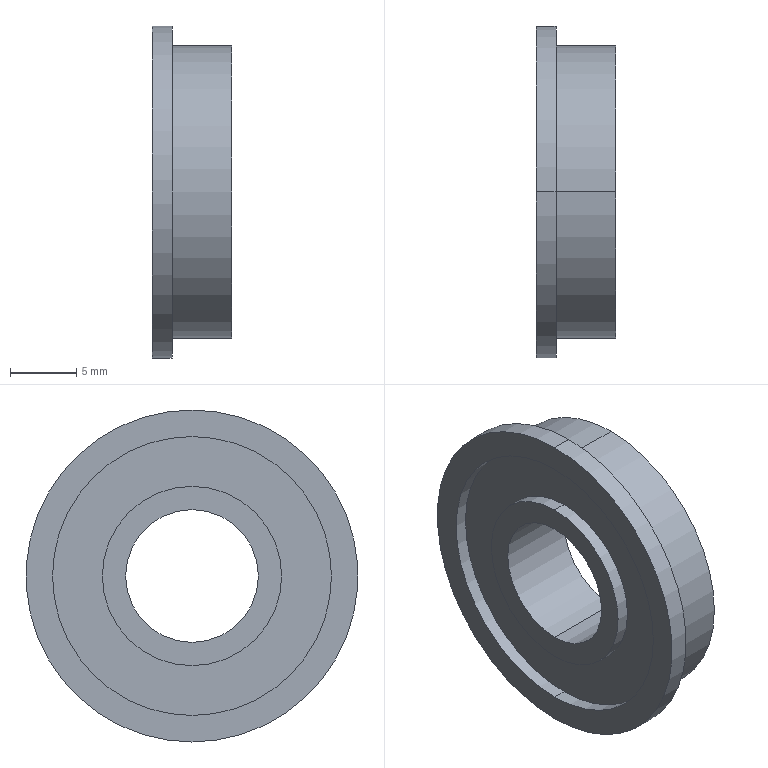Part | SolidWorks | features Stock 1 | 1 solid | 21 faces | box 6 x 25 x 25 mm | volume 1569 mm3 | cylinder 14 | plane 7 | commonest cylinder face diameters 13.5 x4 21 x4 10 x2 22 x2 25 x2
STEP:
#1=CARTESIAN_POINT('',(1.,0.,6.75));
#2=VERTEX_POINT('',#1);
#3=CARTESIAN_POINT('',(1.,0.,-6.75));
#4=VERTEX_POINT('',#3);
#5=CARTESIAN_POINT('',(1.,0.,0.));
#6=DIRECTION('',(-1.,0.,0.));
#7=DIRECTION('',(0.,0.,1.));
#8=AXIS2_PLACEMENT_3D('',#5,#6,#7);
#9=CIRCLE('',#8,6.75);
#10=EDGE_CURVE('',#2,#4,#9,.T.);
#11=ORIENTED_EDGE('',*,*,#10,.T.);
#12=CARTESIAN_POINT('',(0.,0.,-6.75));
#13=VERTEX_POINT('',#12);
#14=CARTESIAN_POINT('',(1.,0.,-6.75));
#15=DIRECTION('',(-1.,0.,0.));
#16=VECTOR('',#15,1000.);
#17=LINE('',#14,#16);
#18=EDGE_CURVE('',#4,#13,#17,.T.);
#19=ORIENTED_EDGE('',*,*,#18,.T.);
#20=CARTESIAN_POINT('',(0.,0.,6.75));
#21=VERTEX_POINT('',#20);
#22=CARTESIAN_POINT('',(0.,0.,0.));
#23=DIRECTION('',(-1.,0.,0.));
#24=DIRECTION('',(0.,0.,1.));
#25=AXIS2_PLACEMENT_3D('',#22,#23,#24);
#26=CIRCLE('',#25,6.75);
#27=EDGE_CURVE('',#21,#13,#26,.T.);
#28=ORIENTED_EDGE('',*,*,#27,.F.);
#29=CARTESIAN_POINT('',(1.,0.,6.75));
#30=DIRECTION('',(-1.,0.,0.));
#31=VECTOR('',#30,1000.);
#32=LINE('',#29,#31);
#33=EDGE_CURVE('',#2,#21,#32,.T.);
#34=ORIENTED_EDGE('',*,*,#33,.F.);
#35=EDGE_LOOP('',(#11,#19,#28,#34));
#36=FACE_OUTER_BOUND('',#35,.T.);
#37=CARTESIAN_POINT('',(1.,0.,0.));
#38=DIRECTION('',(-1.,0.,0.));
#39=DIRECTION('',(0.,0.,1.));
#40=AXIS2_PLACEMENT_3D('',#37,#38,#39);
#41=CYLINDRICAL_SURFACE('',#40,6.75);
#42=ADVANCED_FACE('',(#36),#41,.T.);
#43=CARTESIAN_POINT('',(1.,0.,-10.5));
#44=VERTEX_POINT('',#43);
#45=CARTESIAN_POINT('',(1.,0.,10.5));
#46=VERTEX_POINT('',#45);
#47=CARTESIAN_POINT('',(1.,0.,0.));
#48=DIRECTION('',(-1.,0.,0.));
#49=DIRECTION('',(0.,0.,1.));
#50=AXIS2_PLACEMENT_3D('',#47,#48,#49);
#51=CIRCLE('',#50,10.5);
#52=EDGE_CURVE('',#44,#46,#51,.T.);
#53=ORIENTED_EDGE('',*,*,#52,.F.);
#54=CARTESIAN_POINT('',(0.,0.,-10.5));
#55=VERTEX_POINT('',#54);
#56=CARTESIAN_POINT('',(1.,0.,-10.5));
#57=DIRECTION('',(-1.,0.,0.));
#58=VECTOR('',#57,1000.);
#59=LINE('',#56,#58);
#60=EDGE_CURVE('',#44,#55,#59,.T.);
#61=ORIENTED_EDGE('',*,*,#60,.T.);
#62=CARTESIAN_POINT('',(0.,0.,10.5));
#63=VERTEX_POINT('',#62);
#64=CARTESIAN_POINT('',(0.,0.,0.));
#65=DIRECTION('',(-1.,0.,0.));
#66=DIRECTION('',(0.,0.,1.));
#67=AXIS2_PLACEMENT_3D('',#64,#65,#66);
#68=CIRCLE('',#67,10.5);
#69=EDGE_CURVE('',#55,#63,#68,.T.);
#70=ORIENTED_EDGE('',*,*,#69,.T.);
#71=CARTESIAN_POINT('',(1.,0.,10.5));
#72=DIRECTION('',(-1.,0.,0.));
#73=VECTOR('',#72,1000.);
#74=LINE('',#71,#73);
#75=EDGE_CURVE('',#46,#63,#74,.T.);
#76=ORIENTED_EDGE('',*,*,#75,.F.);
#77=EDGE_LOOP('',(#53,#61,#70,#76));
#78=FACE_OUTER_BOUND('',#77,.T.);
#79=CARTESIAN_POINT('',(1.,0.,0.));
#80=DIRECTION('',(-1.,0.,0.));
#81=DIRECTION('',(0.,0.,1.));
#82=AXIS2_PLACEMENT_3D('',#79,#80,#81);
#83=CYLINDRICAL_SURFACE('',#82,10.5);
#84=ADVANCED_FACE('',(#78),#83,.F.);
#85=CARTESIAN_POINT('',(5.,0.,-6.75));
#86=VERTEX_POINT('',#85);
#87=CARTESIAN_POINT('',(5.,0.,6.75));
#88=VERTEX_POINT('',#87);
#89=CARTESIAN_POINT('',(5.,0.,0.));
#90=DIRECTION('',(1.,0.,0.));
#91=DIRECTION('',(0.,0.,-1.));
#92=AXIS2_PLACEMENT_3D('',#89,#90,#91);
#93=CIRCLE('',#92,6.75);
#94=EDGE_CURVE('',#86,#88,#93,.T.);
#95=ORIENTED_EDGE('',*,*,#94,.T.);
#96=CARTESIAN_POINT('',(6.,0.,6.75));
#97=VERTEX_POINT('',#96);
#98=CARTESIAN_POINT('',(5.,0.,6.75));
#99=DIRECTION('',(1.,0.,0.));
#100=VECTOR('',#99,1000.);
#101=LINE('',#98,#100);
#102=EDGE_CURVE('',#88,#97,#101,.T.);
#103=ORIENTED_EDGE('',*,*,#102,.T.);
#104=CARTESIAN_POINT('',(6.,0.,-6.75));
#105=VERTEX_POINT('',#104);
#106=CARTESIAN_POINT('',(6.,0.,0.));
#107=DIRECTION('',(1.,0.,0.));
#108=DIRECTION('',(0.,0.,-1.));
#109=AXIS2_PLACEMENT_3D('',#106,#107,#108);
#110=CIRCLE('',#109,6.75);
#111=EDGE_CURVE('',#105,#97,#110,.T.);
#112=ORIENTED_EDGE('',*,*,#111,.F.);
#113=CARTESIAN_POINT('',(5.,0.,-6.75));
#114=DIRECTION('',(1.,0.,0.));
#115=VECTOR('',#114,1000.);
#116=LINE('',#113,#115);
#117=EDGE_CURVE('',#86,#105,#116,.T.);
#118=ORIENTED_EDGE('',*,*,#117,.F.);
#119=EDGE_LOOP('',(#95,#103,#112,#118));
#120=FACE_OUTER_BOUND('',#119,.T.);
#121=CARTESIAN_POINT('',(5.,0.,0.));
#122=DIRECTION('',(1.,0.,0.));
#123=DIRECTION('',(0.,0.,-1.));
#124=AXIS2_PLACEMENT_3D('',#121,#122,#123);
#125=CYLINDRICAL_SURFACE('',#124,6.75);
#126=ADVANCED_FACE('',(#120),#125,.T.);
#127=CARTESIAN_POINT('',(5.,0.,10.5));
#128=VERTEX_POINT('',#127);
#129=CARTESIAN_POINT('',(5.,0.,-10.5));
#130=VERTEX_POINT('',#129);
#131=CARTESIAN_POINT('',(5.,0.,0.));
#132=DIRECTION('',(1.,0.,0.));
#133=DIRECTION('',(0.,0.,-1.));
#134=AXIS2_PLACEMENT_3D('',#131,#132,#133);
#135=CIRCLE('',#134,10.5);
#136=EDGE_CURVE('',#128,#130,#135,.T.);
#137=ORIENTED_EDGE('',*,*,#136,.F.);
#138=CARTESIAN_POINT('',(6.,0.,10.5));
#139=VERTEX_POINT('',#138);
#140=CARTESIAN_POINT('',(5.,0.,10.5));
#141=DIRECTION('',(1.,0.,0.));
#142=VECTOR('',#141,1000.);
#143=LINE('',#140,#142);
#144=EDGE_CURVE('',#128,#139,#143,.T.);
#145=ORIENTED_EDGE('',*,*,#144,.T.);
#146=CARTESIAN_POINT('',(6.,0.,-10.5));
#147=VERTEX_POINT('',#146);
#148=CARTESIAN_POINT('',(6.,0.,0.));
#149=DIRECTION('',(1.,0.,0.));
#150=DIRECTION('',(0.,0.,-1.));
#151=AXIS2_PLACEMENT_3D('',#148,#149,#150);
#152=CIRCLE('',#151,10.5);
#153=EDGE_CURVE('',#139,#147,#152,.T.);
#154=ORIENTED_EDGE('',*,*,#153,.T.);
#155=CARTESIAN_POINT('',(5.,0.,-10.5));
#156=DIRECTION('',(1.,0.,0.));
#157=VECTOR('',#156,1000.);
#158=LINE('',#155,#157);
#159=EDGE_CURVE('',#130,#147,#158,.T.);
#160=ORIENTED_EDGE('',*,*,#159,.F.);
#161=EDGE_LOOP('',(#137,#145,#154,#160));
#162=FACE_OUTER_BOUND('',#161,.T.);
#163=CARTESIAN_POINT('',(5.,0.,0.));
#164=DIRECTION('',(1.,0.,0.));
#165=DIRECTION('',(0.,0.,-1.));
#166=AXIS2_PLACEMENT_3D('',#163,#164,#165);
#167=CYLINDRICAL_SURFACE('',#166,10.5);
#168=ADVANCED_FACE('',(#162),#167,.F.);
#169=CARTESIAN_POINT('',(1.5,0.,12.5));
#170=VERTEX_POINT('',#169);
#171=CARTESIAN_POINT('',(1.5,0.,-12.5));
#172=VERTEX_POINT('',#171);
#173=CARTESIAN_POINT('',(1.5,0.,0.));
#174=DIRECTION('',(-1.,0.,0.));
#175=DIRECTION('',(0.,0.,1.));
#176=AXIS2_PLACEMENT_3D('',#173,#174,#175);
#177=CIRCLE('',#176,12.5);
#178=EDGE_CURVE('',#170,#172,#177,.T.);
#179=ORIENTED_EDGE('',*,*,#178,.T.);
#180=CARTESIAN_POINT('',(0.,0.,-12.5));
#181=VERTEX_POINT('',#180);
#182=CARTESIAN_POINT('',(0.,0.,-12.5));
#183=DIRECTION('',(-1.,0.,0.));
#184=VECTOR('',#183,1000.);
#185=LINE('',#182,#184);
#186=EDGE_CURVE('',#172,#181,#185,.T.);
#187=ORIENTED_EDGE('',*,*,#186,.T.);
#188=CARTESIAN_POINT('',(0.,0.,12.5));
#189=VERTEX_POINT('',#188);
#190=CARTESIAN_POINT('',(0.,0.,0.));
#191=DIRECTION('',(-1.,0.,0.));
#192=DIRECTION('',(0.,0.,1.));
#193=AXIS2_PLACEMENT_3D('',#190,#191,#192);
#194=CIRCLE('',#193,12.5);
#195=EDGE_CURVE('',#189,#181,#194,.T.);
#196=ORIENTED_EDGE('',*,*,#195,.F.);
#197=CARTESIAN_POINT('',(0.,0.,12.5));
#198=DIRECTION('',(-1.,0.,0.));
#199=VECTOR('',#198,1000.);
#200=LINE('',#197,#199);
#201=EDGE_CURVE('',#170,#189,#200,.T.);
#202=ORIENTED_EDGE('',*,*,#201,.F.);
#203=EDGE_LOOP('',(#179,#187,#196,#202));
#204=FACE_OUTER_BOUND('',#203,.T.);
#205=CARTESIAN_POINT('',(0.,0.,0.));
#206=DIRECTION('',(-1.,0.,0.));
#207=DIRECTION('',(0.,0.,1.));
#208=AXIS2_PLACEMENT_3D('',#205,#206,#207);
#209=CYLINDRICAL_SURFACE('',#208,12.5);
#210=ADVANCED_FACE('',(#204),#209,.T.);
#211=CARTESIAN_POINT('',(6.,0.,11.));
#212=VERTEX_POINT('',#211);
#213=CARTESIAN_POINT('',(6.,0.,-11.));
#214=VERTEX_POINT('',#213);
#215=CARTESIAN_POINT('',(6.,0.,0.));
#216=DIRECTION('',(-1.,0.,0.));
#217=DIRECTION('',(0.,0.,1.));
#218=AXIS2_PLACEMENT_3D('',#215,#216,#217);
#219=CIRCLE('',#218,11.);
#220=EDGE_CURVE('',#212,#214,#219,.T.);
#221=ORIENTED_EDGE('',*,*,#220,.T.);
#222=CARTESIAN_POINT('',(1.5,0.,-11.));
#223=VERTEX_POINT('',#222);
#224=CARTESIAN_POINT('',(0.,0.,-11.));
#225=DIRECTION('',(-1.,0.,0.));
#226=VECTOR('',#225,1000.);
#227=LINE('',#224,#226);
#228=EDGE_CURVE('',#214,#223,#227,.T.);
#229=ORIENTED_EDGE('',*,*,#228,.T.);
#230=CARTESIAN_POINT('',(1.5,0.,11.));
#231=VERTEX_POINT('',#230);
#232=CARTESIAN_POINT('',(1.5,0.,0.));
#233=DIRECTION('',(-1.,0.,0.));
#234=DIRECTION('',(0.,0.,1.));
#235=AXIS2_PLACEMENT_3D('',#232,#233,#234);
#236=CIRCLE('',#235,11.);
#237=EDGE_CURVE('',#231,#223,#236,.T.);
#238=ORIENTED_EDGE('',*,*,#237,.F.);
#239=CARTESIAN_POINT('',(0.,0.,11.));
#240=DIRECTION('',(-1.,0.,0.));
#241=VECTOR('',#240,1000.);
#242=LINE('',#239,#241);
#243=EDGE_CURVE('',#212,#231,#242,.T.);
#244=ORIENTED_EDGE('',*,*,#243,.F.);
#245=EDGE_LOOP('',(#221,#229,#238,#244));
#246=FACE_OUTER_BOUND('',#245,.T.);
#247=CARTESIAN_POINT('',(0.,0.,0.));
#248=DIRECTION('',(-1.,0.,0.));
#249=DIRECTION('',(0.,0.,1.));
#250=AXIS2_PLACEMENT_3D('',#247,#248,#249);
#251=CYLINDRICAL_SURFACE('',#250,11.);
#252=ADVANCED_FACE('',(#246),#251,.T.);
#253=CARTESIAN_POINT('',(6.,0.,-5.));
#254=VERTEX_POINT('',#253);
#255=CARTESIAN_POINT('',(6.,0.,5.));
#256=VERTEX_POINT('',#255);
#257=CARTESIAN_POINT('',(6.,0.,0.));
#258=DIRECTION('',(-1.,0.,0.));
#259=DIRECTION('',(0.,0.,1.));
#260=AXIS2_PLACEMENT_3D('',#257,#258,#259);
#261=CIRCLE('',#260,5.);
#262=EDGE_CURVE('',#254,#256,#261,.T.);
#263=ORIENTED_EDGE('',*,*,#262,.F.);
#264=CARTESIAN_POINT('',(0.,0.,-5.));
#265=VERTEX_POINT('',#264);
#266=CARTESIAN_POINT('',(0.,0.,-5.));
#267=DIRECTION('',(-1.,0.,0.));
#268=VECTOR('',#267,1000.);
#269=LINE('',#266,#268);
#270=EDGE_CURVE('',#254,#265,#269,.T.);
#271=ORIENTED_EDGE('',*,*,#270,.T.);
#272=CARTESIAN_POINT('',(0.,0.,5.));
#273=VERTEX_POINT('',#272);
#274=CARTESIAN_POINT('',(0.,0.,0.));
#275=DIRECTION('',(-1.,0.,0.));
#276=DIRECTION('',(0.,0.,1.));
#277=AXIS2_PLACEMENT_3D('',#274,#275,#276);
#278=CIRCLE('',#277,5.);
#279=EDGE_CURVE('',#265,#273,#278,.T.);
#280=ORIENTED_EDGE('',*,*,#279,.T.);
#281=CARTESIAN_POINT('',(0.,0.,5.));
#282=DIRECTION('',(-1.,0.,0.));
#283=VECTOR('',#282,1000.);
#284=LINE('',#281,#283);
#285=EDGE_CURVE('',#256,#273,#284,.T.);
#286=ORIENTED_EDGE('',*,*,#285,.F.);
#287=EDGE_LOOP('',(#263,#271,#280,#286));
#288=FACE_OUTER_BOUND('',#287,.T.);
#289=CARTESIAN_POINT('',(0.,0.,0.));
#290=DIRECTION('',(-1.,0.,0.));
#291=DIRECTION('',(0.,0.,1.));
#292=AXIS2_PLACEMENT_3D('',#289,#290,#291);
#293=CYLINDRICAL_SURFACE('',#292,5.);
#294=ADVANCED_FACE('',(#288),#293,.F.);
#295=CARTESIAN_POINT('',(0.,0.,0.));
#296=DIRECTION('',(-1.,0.,0.));
#297=DIRECTION('',(0.,0.,1.));
#298=AXIS2_PLACEMENT_3D('',#295,#296,#297);
#299=CIRCLE('',#298,5.);
#300=EDGE_CURVE('',#273,#265,#299,.T.);
#301=ORIENTED_EDGE('',*,*,#300,.F.);
#302=ORIENTED_EDGE('',*,*,#279,.F.);
#303=EDGE_LOOP('',(#301,#302));
#304=FACE_BOUND('',#303,.T.);
#305=ORIENTED_EDGE('',*,*,#27,.T.);
#306=CARTESIAN_POINT('',(0.,0.,0.));
#307=DIRECTION('',(-1.,0.,0.));
#308=DIRECTION('',(0.,0.,1.));
#309=AXIS2_PLACEMENT_3D('',#306,#307,#308);
#310=CIRCLE('',#309,6.75);
#311=EDGE_CURVE('',#13,#21,#310,.T.);
#312=ORIENTED_EDGE('',*,*,#311,.T.);
#313=EDGE_LOOP('',(#305,#312));
#314=FACE_OUTER_BOUND('',#313,.T.);
#315=CARTESIAN_POINT('',(0.,0.,0.));
#316=DIRECTION('',(1.,0.,0.));
#317=DIRECTION('',(0.,0.,-1.));
#318=AXIS2_PLACEMENT_3D('',#315,#316,#317);
#319=PLANE('',#318);
#320=ADVANCED_FACE('',(#304,#314),#319,.F.);
#321=CARTESIAN_POINT('',(6.,0.,0.));
#322=DIRECTION('',(-1.,0.,0.));
#323=DIRECTION('',(0.,0.,1.));
#324=AXIS2_PLACEMENT_3D('',#321,#322,#323);
#325=CIRCLE('',#324,5.);
#326=EDGE_CURVE('',#256,#254,#325,.T.);
#327=ORIENTED_EDGE('',*,*,#326,.T.);
#328=ORIENTED_EDGE('',*,*,#262,.T.);
#329=EDGE_LOOP('',(#327,#328));
#330=FACE_BOUND('',#329,.T.);
#331=ORIENTED_EDGE('',*,*,#111,.T.);
#332=CARTESIAN_POINT('',(6.,0.,0.));
#333=DIRECTION('',(1.,0.,0.));
#334=DIRECTION('',(0.,0.,-1.));
#335=AXIS2_PLACEMENT_3D('',#332,#333,#334);
#336=CIRCLE('',#335,6.75);
#337=EDGE_CURVE('',#97,#105,#336,.T.);
#338=ORIENTED_EDGE('',*,*,#337,.T.);
#339=EDGE_LOOP('',(#331,#338));
#340=FACE_OUTER_BOUND('',#339,.T.);
#341=CARTESIAN_POINT('',(6.,0.,0.));
#342=DIRECTION('',(-1.,0.,0.));
#343=DIRECTION('',(0.,0.,1.));
#344=AXIS2_PLACEMENT_3D('',#341,#342,#343);
#345=PLANE('',#344);
#346=ADVANCED_FACE('',(#330,#340),#345,.F.);
#347=CARTESIAN_POINT('',(0.,0.,0.));
#348=DIRECTION('',(-1.,0.,0.));
#349=DIRECTION('',(0.,0.,1.));
#350=AXIS2_PLACEMENT_3D('',#347,#348,#349);
#351=CIRCLE('',#350,10.5);
#352=EDGE_CURVE('',#63,#55,#351,.T.);
#353=ORIENTED_EDGE('',*,*,#352,.F.);
#354=ORIENTED_EDGE('',*,*,#69,.F.);
#355=EDGE_LOOP('',(#353,#354));
#356=FACE_BOUND('',#355,.T.);
#357=ORIENTED_EDGE('',*,*,#195,.T.);
#358=CARTESIAN_POINT('',(0.,0.,0.));
#359=DIRECTION('',(-1.,0.,0.));
#360=DIRECTION('',(0.,0.,1.));
#361=AXIS2_PLACEMENT_3D('',#358,#359,#360);
#362=CIRCLE('',#361,12.5);
#363=EDGE_CURVE('',#181,#189,#362,.T.);
#364=ORIENTED_EDGE('',*,*,#363,.T.);
#365=EDGE_LOOP('',(#357,#364));
#366=FACE_OUTER_BOUND('',#365,.T.);
#367=CARTESIAN_POINT('',(0.,0.,0.));
#368=DIRECTION('',(1.,0.,0.));
#369=DIRECTION('',(0.,0.,-1.));
#370=AXIS2_PLACEMENT_3D('',#367,#368,#369);
#371=PLANE('',#370);
#372=ADVANCED_FACE('',(#356,#366),#371,.F.);
#373=ORIENTED_EDGE('',*,*,#270,.F.);
#374=ORIENTED_EDGE('',*,*,#326,.F.);
#375=ORIENTED_EDGE('',*,*,#285,.T.);
#376=ORIENTED_EDGE('',*,*,#300,.T.);
#377=EDGE_LOOP('',(#373,#374,#375,#376));
#378=FACE_OUTER_BOUND('',#377,.T.);
#379=CARTESIAN_POINT('',(0.,0.,0.));
#380=DIRECTION('',(-1.,0.,0.));
#381=DIRECTION('',(0.,0.,1.));
#382=AXIS2_PLACEMENT_3D('',#379,#380,#381);
#383=CYLINDRICAL_SURFACE('',#382,5.);
#384=ADVANCED_FACE('',(#378),#383,.F.);
#385=CARTESIAN_POINT('',(6.,0.,0.));
#386=DIRECTION('',(1.,0.,0.));
#387=DIRECTION('',(0.,0.,-1.));
#388=AXIS2_PLACEMENT_3D('',#385,#386,#387);
#389=CIRCLE('',#388,10.5);
#390=EDGE_CURVE('',#147,#139,#389,.T.);
#391=ORIENTED_EDGE('',*,*,#390,.F.);
#392=ORIENTED_EDGE('',*,*,#153,.F.);
#393=EDGE_LOOP('',(#391,#392));
#394=FACE_BOUND('',#393,.T.);
#395=ORIENTED_EDGE('',*,*,#220,.F.);
#396=CARTESIAN_POINT('',(6.,0.,0.));
#397=DIRECTION('',(-1.,0.,0.));
#398=DIRECTION('',(0.,0.,1.));
#399=AXIS2_PLACEMENT_3D('',#396,#397,#398);
#400=CIRCLE('',#399,11.);
#401=EDGE_CURVE('',#214,#212,#400,.T.);
#402=ORIENTED_EDGE('',*,*,#401,.F.);
#403=EDGE_LOOP('',(#395,#402));
#404=FACE_OUTER_BOUND('',#403,.T.);
#405=CARTESIAN_POINT('',(6.,0.,0.));
#406=DIRECTION('',(-1.,0.,0.));
#407=DIRECTION('',(0.,0.,1.));
#408=AXIS2_PLACEMENT_3D('',#405,#406,#407);
#409=PLANE('',#408);
#410=ADVANCED_FACE('',(#394,#404),#409,.F.);
#411=ORIENTED_EDGE('',*,*,#228,.F.);
#412=ORIENTED_EDGE('',*,*,#401,.T.);
#413=ORIENTED_EDGE('',*,*,#243,.T.);
#414=CARTESIAN_POINT('',(1.5,0.,0.));
#415=DIRECTION('',(-1.,0.,0.));
#416=DIRECTION('',(0.,0.,1.));
#417=AXIS2_PLACEMENT_3D('',#414,#415,#416);
#418=CIRCLE('',#417,11.);
#419=EDGE_CURVE('',#223,#231,#418,.T.);
#420=ORIENTED_EDGE('',*,*,#419,.F.);
#421=EDGE_LOOP('',(#411,#412,#413,#420));
#422=FACE_OUTER_BOUND('',#421,.T.);
#423=CARTESIAN_POINT('',(0.,0.,0.));
#424=DIRECTION('',(-1.,0.,0.));
#425=DIRECTION('',(0.,0.,1.));
#426=AXIS2_PLACEMENT_3D('',#423,#424,#425);
#427=CYLINDRICAL_SURFACE('',#426,11.);
#428=ADVANCED_FACE('',(#422),#427,.T.);
#429=ORIENTED_EDGE('',*,*,#178,.F.);
#430=CARTESIAN_POINT('',(1.5,0.,0.));
#431=DIRECTION('',(-1.,0.,0.));
#432=DIRECTION('',(0.,0.,1.));
#433=AXIS2_PLACEMENT_3D('',#430,#431,#432);
#434=CIRCLE('',#433,12.5);
#435=EDGE_CURVE('',#172,#170,#434,.T.);
#436=ORIENTED_EDGE('',*,*,#435,.F.);
#437=EDGE_LOOP('',(#429,#436));
#438=FACE_OUTER_BOUND('',#437,.T.);
#439=ORIENTED_EDGE('',*,*,#237,.T.);
#440=ORIENTED_EDGE('',*,*,#419,.T.);
#441=EDGE_LOOP('',(#439,#440));
#442=FACE_BOUND('',#441,.T.);
#443=CARTESIAN_POINT('',(1.5,0.,0.));
#444=DIRECTION('',(-1.,0.,0.));
#445=DIRECTION('',(0.,0.,1.));
#446=AXIS2_PLACEMENT_3D('',#443,#444,#445);
#447=PLANE('',#446);
#448=ADVANCED_FACE('',(#438,#442),#447,.F.);
#449=ORIENTED_EDGE('',*,*,#186,.F.);
#450=ORIENTED_EDGE('',*,*,#435,.T.);
#451=ORIENTED_EDGE('',*,*,#201,.T.);
#452=ORIENTED_EDGE('',*,*,#363,.F.);
#453=EDGE_LOOP('',(#449,#450,#451,#452));
#454=FACE_OUTER_BOUND('',#453,.T.);
#455=CARTESIAN_POINT('',(0.,0.,0.));
#456=DIRECTION('',(-1.,0.,0.));
#457=DIRECTION('',(0.,0.,1.));
#458=AXIS2_PLACEMENT_3D('',#455,#456,#457);
#459=CYLINDRICAL_SURFACE('',#458,12.5);
#460=ADVANCED_FACE('',(#454),#459,.T.);
#461=ORIENTED_EDGE('',*,*,#144,.F.);
#462=CARTESIAN_POINT('',(5.,0.,0.));
#463=DIRECTION('',(1.,0.,0.));
#464=DIRECTION('',(0.,0.,-1.));
#465=AXIS2_PLACEMENT_3D('',#462,#463,#464);
#466=CIRCLE('',#465,10.5);
#467=EDGE_CURVE('',#130,#128,#466,.T.);
#468=ORIENTED_EDGE('',*,*,#467,.F.);
#469=ORIENTED_EDGE('',*,*,#159,.T.);
#470=ORIENTED_EDGE('',*,*,#390,.T.);
#471=EDGE_LOOP('',(#461,#468,#469,#470));
#472=FACE_OUTER_BOUND('',#471,.T.);
#473=CARTESIAN_POINT('',(5.,0.,0.));
#474=DIRECTION('',(1.,0.,0.));
#475=DIRECTION('',(0.,0.,-1.));
#476=AXIS2_PLACEMENT_3D('',#473,#474,#475);
#477=CYLINDRICAL_SURFACE('',#476,10.5);
#478=ADVANCED_FACE('',(#472),#477,.F.);
#479=ORIENTED_EDGE('',*,*,#94,.F.);
#480=CARTESIAN_POINT('',(5.,0.,0.));
#481=DIRECTION('',(1.,0.,0.));
#482=DIRECTION('',(0.,0.,-1.));
#483=AXIS2_PLACEMENT_3D('',#480,#481,#482);
#484=CIRCLE('',#483,6.75);
#485=EDGE_CURVE('',#88,#86,#484,.T.);
#486=ORIENTED_EDGE('',*,*,#485,.F.);
#487=EDGE_LOOP('',(#479,#486));
#488=FACE_BOUND('',#487,.T.);
#489=ORIENTED_EDGE('',*,*,#467,.T.);
#490=ORIENTED_EDGE('',*,*,#136,.T.);
#491=EDGE_LOOP('',(#489,#490));
#492=FACE_OUTER_BOUND('',#491,.T.);
#493=CARTESIAN_POINT('',(5.,0.,0.));
#494=DIRECTION('',(1.,0.,0.));
#495=DIRECTION('',(0.,0.,-1.));
#496=AXIS2_PLACEMENT_3D('',#493,#494,#495);
#497=PLANE('',#496);
#498=ADVANCED_FACE('',(#488,#492),#497,.T.);
#499=ORIENTED_EDGE('',*,*,#102,.F.);
#500=ORIENTED_EDGE('',*,*,#485,.T.);
#501=ORIENTED_EDGE('',*,*,#117,.T.);
#502=ORIENTED_EDGE('',*,*,#337,.F.);
#503=EDGE_LOOP('',(#499,#500,#501,#502));
#504=FACE_OUTER_BOUND('',#503,.T.);
#505=CARTESIAN_POINT('',(5.,0.,0.));
#506=DIRECTION('',(1.,0.,0.));
#507=DIRECTION('',(0.,0.,-1.));
#508=AXIS2_PLACEMENT_3D('',#505,#506,#507);
#509=CYLINDRICAL_SURFACE('',#508,6.75);
#510=ADVANCED_FACE('',(#504),#509,.T.);
#511=ORIENTED_EDGE('',*,*,#60,.F.);
#512=CARTESIAN_POINT('',(1.,0.,0.));
#513=DIRECTION('',(-1.,0.,0.));
#514=DIRECTION('',(0.,0.,1.));
#515=AXIS2_PLACEMENT_3D('',#512,#513,#514);
#516=CIRCLE('',#515,10.5);
#517=EDGE_CURVE('',#46,#44,#516,.T.);
#518=ORIENTED_EDGE('',*,*,#517,.F.);
#519=ORIENTED_EDGE('',*,*,#75,.T.);
#520=ORIENTED_EDGE('',*,*,#352,.T.);
#521=EDGE_LOOP('',(#511,#518,#519,#520));
#522=FACE_OUTER_BOUND('',#521,.T.);
#523=CARTESIAN_POINT('',(1.,0.,0.));
#524=DIRECTION('',(-1.,0.,0.));
#525=DIRECTION('',(0.,0.,1.));
#526=AXIS2_PLACEMENT_3D('',#523,#524,#525);
#527=CYLINDRICAL_SURFACE('',#526,10.5);
#528=ADVANCED_FACE('',(#522),#527,.F.);
#529=ORIENTED_EDGE('',*,*,#10,.F.);
#530=CARTESIAN_POINT('',(1.,0.,0.));
#531=DIRECTION('',(-1.,0.,0.));
#532=DIRECTION('',(0.,0.,1.));
#533=AXIS2_PLACEMENT_3D('',#530,#531,#532);
#534=CIRCLE('',#533,6.75);
#535=EDGE_CURVE('',#4,#2,#534,.T.);
#536=ORIENTED_EDGE('',*,*,#535,.F.);
#537=EDGE_LOOP('',(#529,#536));
#538=FACE_BOUND('',#537,.T.);
#539=ORIENTED_EDGE('',*,*,#517,.T.);
#540=ORIENTED_EDGE('',*,*,#52,.T.);
#541=EDGE_LOOP('',(#539,#540));
#542=FACE_OUTER_BOUND('',#541,.T.);
#543=CARTESIAN_POINT('',(1.,0.,0.));
#544=DIRECTION('',(-1.,0.,0.));
#545=DIRECTION('',(0.,0.,1.));
#546=AXIS2_PLACEMENT_3D('',#543,#544,#545);
#547=PLANE('',#546);
#548=ADVANCED_FACE('',(#538,#542),#547,.T.);
#549=ORIENTED_EDGE('',*,*,#18,.F.);
#550=ORIENTED_EDGE('',*,*,#535,.T.);
#551=ORIENTED_EDGE('',*,*,#33,.T.);
#552=ORIENTED_EDGE('',*,*,#311,.F.);
#553=EDGE_LOOP('',(#549,#550,#551,#552));
#554=FACE_OUTER_BOUND('',#553,.T.);
#555=CARTESIAN_POINT('',(1.,0.,0.));
#556=DIRECTION('',(-1.,0.,0.));
#557=DIRECTION('',(0.,0.,1.));
#558=AXIS2_PLACEMENT_3D('',#555,#556,#557);
#559=CYLINDRICAL_SURFACE('',#558,6.75);
#560=ADVANCED_FACE('',(#554),#559,.T.);
#561=CLOSED_SHELL('',(#42,#84,#126,#168,#210,#252,#294,#320,#346,#372,#384,#410,#428,#448,#460,#478,#498,#510,#528,#548,#560));
#562=MANIFOLD_SOLID_BREP('',#561);
#563=CARTESIAN_POINT('',(0.,0.,0.));
#564=DIRECTION('',(0.,0.,1.));
#565=DIRECTION('',(1.,0.,0.));
#566=AXIS2_PLACEMENT_3D('',#563,#564,#565);
#567=(LENGTH_UNIT()NAMED_UNIT(*)SI_UNIT(.MILLI.,.METRE.));
#568=UNCERTAINTY_MEASURE_WITH_UNIT(LENGTH_MEASURE(0.00001),#567,'','');
#569=(NAMED_UNIT(*)PLANE_ANGLE_UNIT()SI_UNIT($,.RADIAN.));
#570=(NAMED_UNIT(*)SI_UNIT($,.STERADIAN.)SOLID_ANGLE_UNIT());
#571=(GEOMETRIC_REPRESENTATION_CONTEXT(3)GLOBAL_UNCERTAINTY_ASSIGNED_CONTEXT((#568))GLOBAL_UNIT_ASSIGNED_CONTEXT((#567,#569,#570))REPRESENTATION_CONTEXT('',''));
#572=ADVANCED_BREP_SHAPE_REPRESENTATION('',(#562,#566),#571);